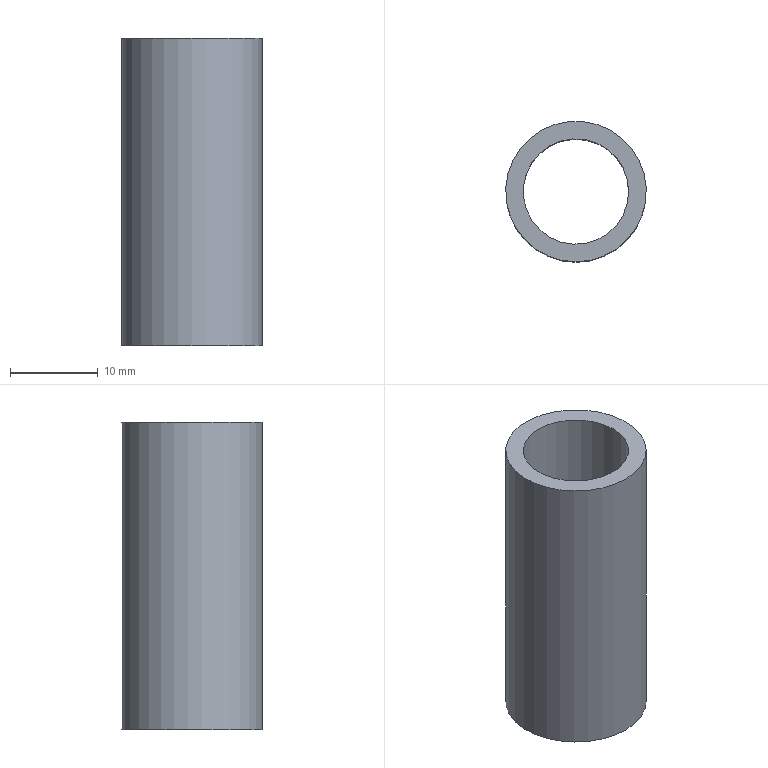Part | NX | features solid 2 | 1 solid | 4 faces | box 16 x 16 x 35 mm | volume 3079 mm3 | plane 2 | cylinder 2 | commonest cylinder face diameters 12 x1 16 x1
STEP:
#1=CARTESIAN_POINT('',(-108.783,425.511,-30.));
#2=VERTEX_POINT('',#1);
#3=CARTESIAN_POINT('',(-114.783,425.511,-30.));
#4=DIRECTION('',(0.,0.,1.));
#5=DIRECTION('',(1.,0.,0.));
#6=AXIS2_PLACEMENT_3D('',#3,#4,#5);
#7=CIRCLE('',#6,6.);
#8=EDGE_CURVE('',#2,#2,#7,.F.);
#9=ORIENTED_EDGE('',*,*,#8,.T.);
#10=EDGE_LOOP('',(#9));
#11=FACE_BOUND('',#10,.T.);
#12=CARTESIAN_POINT('',(-114.783,417.511,-30.));
#13=VERTEX_POINT('',#12);
#14=CARTESIAN_POINT('',(-114.783,425.511,-30.));
#15=DIRECTION('',(0.,0.,-1.));
#16=DIRECTION('',(0.,-1.,0.));
#17=AXIS2_PLACEMENT_3D('',#14,#15,#16);
#18=CIRCLE('',#17,8.);
#19=EDGE_CURVE('',#13,#13,#18,.T.);
#20=ORIENTED_EDGE('',*,*,#19,.F.);
#21=EDGE_LOOP('',(#20));
#22=FACE_BOUND('',#21,.T.);
#23=CARTESIAN_POINT('',(-114.783,425.511,-30.));
#24=DIRECTION('',(0.,0.,1.));
#25=DIRECTION('',(1.,0.,0.));
#26=AXIS2_PLACEMENT_3D('',#23,#24,#25);
#27=PLANE('',#26);
#28=ADVANCED_FACE('',(#11,#22),#27,.T.);
#29=CARTESIAN_POINT('',(-108.783,425.511,-65.));
#30=VERTEX_POINT('',#29);
#31=CARTESIAN_POINT('',(-114.783,425.511,-65.));
#32=DIRECTION('',(0.,0.,1.));
#33=DIRECTION('',(1.,0.,0.));
#34=AXIS2_PLACEMENT_3D('',#31,#32,#33);
#35=CIRCLE('',#34,6.);
#36=EDGE_CURVE('',#30,#30,#35,.F.);
#37=ORIENTED_EDGE('',*,*,#36,.F.);
#38=EDGE_LOOP('',(#37));
#39=FACE_BOUND('',#38,.T.);
#40=CARTESIAN_POINT('',(-114.783,417.511,-65.));
#41=VERTEX_POINT('',#40);
#42=CARTESIAN_POINT('',(-114.783,425.511,-65.));
#43=DIRECTION('',(0.,0.,-1.));
#44=DIRECTION('',(0.,-1.,0.));
#45=AXIS2_PLACEMENT_3D('',#42,#43,#44);
#46=CIRCLE('',#45,8.);
#47=EDGE_CURVE('',#41,#41,#46,.T.);
#48=ORIENTED_EDGE('',*,*,#47,.T.);
#49=EDGE_LOOP('',(#48));
#50=FACE_BOUND('',#49,.T.);
#51=CARTESIAN_POINT('',(-114.783,425.511,-65.));
#52=DIRECTION('',(0.,0.,1.));
#53=DIRECTION('',(1.,0.,0.));
#54=AXIS2_PLACEMENT_3D('',#51,#52,#53);
#55=PLANE('',#54);
#56=ADVANCED_FACE('',(#39,#50),#55,.F.);
#57=ORIENTED_EDGE('',*,*,#8,.F.);
#58=EDGE_LOOP('',(#57));
#59=FACE_BOUND('',#58,.T.);
#60=ORIENTED_EDGE('',*,*,#36,.T.);
#61=EDGE_LOOP('',(#60));
#62=FACE_BOUND('',#61,.T.);
#63=CARTESIAN_POINT('',(-114.783,425.511,-65.));
#64=DIRECTION('',(0.,0.,1.));
#65=DIRECTION('',(1.,0.,0.));
#66=AXIS2_PLACEMENT_3D('',#63,#64,#65);
#67=CYLINDRICAL_SURFACE('',#66,6.);
#68=ADVANCED_FACE('',(#59,#62),#67,.F.);
#69=ORIENTED_EDGE('',*,*,#19,.T.);
#70=EDGE_LOOP('',(#69));
#71=FACE_BOUND('',#70,.T.);
#72=ORIENTED_EDGE('',*,*,#47,.F.);
#73=EDGE_LOOP('',(#72));
#74=FACE_BOUND('',#73,.T.);
#75=CARTESIAN_POINT('',(-114.783,425.511,-65.));
#76=DIRECTION('',(0.,0.,1.));
#77=DIRECTION('',(1.,0.,0.));
#78=AXIS2_PLACEMENT_3D('',#75,#76,#77);
#79=CYLINDRICAL_SURFACE('',#78,8.);
#80=ADVANCED_FACE('',(#71,#74),#79,.T.);
#81=CLOSED_SHELL('',(#28,#56,#68,#80));
#82=MANIFOLD_SOLID_BREP('',#81);
#83=(LENGTH_UNIT()NAMED_UNIT(*)SI_UNIT(.MILLI.,.METRE.));
#84=UNCERTAINTY_MEASURE_WITH_UNIT(LENGTH_MEASURE(0.00001),#83,'','');
#85=(NAMED_UNIT(*)PLANE_ANGLE_UNIT()SI_UNIT($,.RADIAN.));
#86=(NAMED_UNIT(*)SI_UNIT($,.STERADIAN.)SOLID_ANGLE_UNIT());
#87=(GEOMETRIC_REPRESENTATION_CONTEXT(3)GLOBAL_UNCERTAINTY_ASSIGNED_CONTEXT((#84))GLOBAL_UNIT_ASSIGNED_CONTEXT((#83,#85,#86))REPRESENTATION_CONTEXT('',''));
#88=ADVANCED_BREP_SHAPE_REPRESENTATION('',(#82),#87);